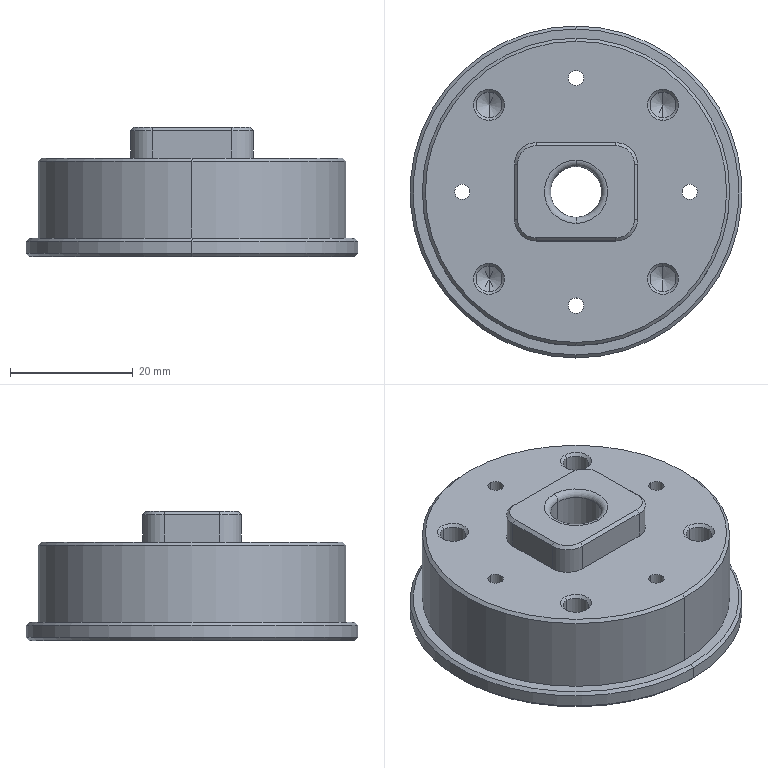NC program | NX | posted with a generic post | part box 54 x 54 x 21 mm
Lines 4215 to 5114 of 9691:
(ZLEVEL_PROFILE_1_COPY , TOOL : D4R0.5)
N8404 T17 M6
N8406 G54
N8408 G17 G0 G90 X-1.092 Y7.723 S9500 M3
N8410 G43 Z30. H17
N8412 Z-0.1
N8414 G94 G1 Z-1.6 F2500.
N8416 X-0.715 Y7.158
N8418 G3 X-0.356 Y6.981 R0.4
N8420 G1 X-0.055 Y7.
N8422 X0.105 Y6.999
N8424 X0.795 Y6.955
N8426 G2 X1.661 Y6.8 R15.853
N8428 G1 X1.824 Y6.758
N8430 X2.491 Y6.542
N8432 X2.656 Y6.477
N8434 X3.299 Y6.174
N8436 X3.391 Y6.123
N8438 X4.045 Y5.713
N8440 X4.129 Y5.652
N8442 X4.719 Y5.17
N8444 X4.804 Y5.091
N8446 X5.336 Y4.531
N8448 X5.445 Y4.399
N8450 X5.865 Y3.821
N8452 G2 X6.711 Y1.978 R7.418
N8454 X6.218 Y-3.201 R6.976
N8456 G1 X5.963 Y-3.665
N8458 G2 X5.445 Y-4.399 R14.342
N8460 G1 X5.37 Y-4.491
N8462 X4.862 Y-5.036
N8464 G2 X4.186 Y-5.611 R8.765
N8466 G1 X4.045 Y-5.713
N8468 X3.455 Y-6.088
N8470 X3.299 Y-6.174
N8472 X2.656 Y-6.477
N8474 X2.544 Y-6.521
N8476 X1.824 Y-6.758
N8478 X1.696 Y-6.791
N8480 X0.972 Y-6.932
N8482 X0.848 Y-6.948
N8484 X0.066 Y-7.
N8486 X-0.088 Y-6.998
N8488 X-0.795 Y-6.955
N8490 G2 X-1.787 Y-6.773 R15.853
N8492 G1 X-1.839 Y-6.752
N8494 X-2.491 Y-6.542
N8496 X-2.656 Y-6.477
N8498 X-3.299 Y-6.174
N8500 X-3.391 Y-6.123
N8502 X-4.045 Y-5.713
N8504 X-4.129 Y-5.652
N8506 X-4.719 Y-5.17
N8508 X-4.804 Y-5.091
N8510 X-5.336 Y-4.531
N8512 X-5.445 Y-4.399
N8514 X-5.855 Y-3.837
N8516 G2 X-6.71 Y-1.978 R7.402
N8518 X-6.218 Y3.202 R6.977
N8520 G1 X-5.963 Y3.665
N8522 G2 X-5.445 Y4.399 R13.396
N8524 G1 X-5.343 Y4.522
N8526 X-4.862 Y5.036
N8528 G2 X-4.186 Y5.611 R8.767
N8530 G1 X-4.045 Y5.713
N8532 X-3.455 Y6.088
N8534 X-3.299 Y6.174
N8536 X-2.656 Y6.477
N8538 X-2.544 Y6.521
N8540 X-1.824 Y6.758
N8542 X-1.696 Y6.791
N8544 X-0.972 Y6.932
N8546 X-0.848 Y6.948
N8548 X-0.356 Y6.981
N8550 X-0.22 Y6.991 Z-1.602
N8552 X-0.084 Y6.999 Z-1.605
N8554 X0.053 Z-1.607
N8556 X0.189 Y6.993 Z-1.61
N8558 X0.325 Y6.984 Z-1.612
N8560 X0.461 Y6.975 Z-1.614
N8562 X0.597 Y6.967 Z-1.617
N8564 X0.733 Y6.958 Z-1.619
N8566 X0.869 Y6.946 Z-1.621
N8568 X1.004 Y6.925 Z-1.624
N8570 X1.138 Y6.899 Z-1.626
N8572 X1.272 Y6.874 Z-1.629
N8574 X1.406 Y6.848 Z-1.631
N8576 X1.54 Y6.823 Z-1.633
N8578 X1.674 Y6.796 Z-1.636
N8580 X1.806 Y6.762 Z-1.638
N8582 X1.936 Y6.721 Z-1.64
N8584 X2.066 Y6.679 Z-1.643
N8586 X2.195 Y6.637 Z-1.645
N8588 X2.325 Y6.595 Z-1.648
N8590 X2.455 Y6.553 Z-1.65
N8592 X2.583 Y6.506 Z-1.652
N8594 X2.708 Y6.452 Z-1.655
N8596 X2.831 Y6.394 Z-1.657
N8598 X2.955 Y6.335 Z-1.66
N8600 X3.078 Y6.278 Z-1.662
N8602 X3.202 Y6.219 Z-1.664
N8604 X3.324 Y6.16 Z-1.667
N8606 X3.444 Y6.094 Z-1.669
N8608 X3.559 Y6.021 Z-1.671
N8610 X3.674 Y5.948 Z-1.674
N8612 X3.789 Y5.875 Z-1.676
N8614 X3.905 Y5.802 Z-1.679
N8616 X4.02 Y5.729 Z-1.681
N8618 X4.131 Y5.65 Z-1.683
N8620 X4.239 Y5.566 Z-1.686
N8622 X4.344 Y5.479 Z-1.688
N8624 X4.449 Y5.392 Z-1.69
N8626 X4.554 Y5.305 Z-1.693
N8628 X4.659 Y5.219 Z-1.695
N8630 X4.763 Y5.13 Z-1.698
N8632 X4.859 Y5.033 Z-1.7
N8634 X5.336 Y4.531
N8636 X5.445 Y4.399
N8638 X5.865 Y3.821
N8640 G2 X6.711 Y1.978 R7.414
N8642 X6.218 Y-3.202 R6.972
N8644 G1 X5.963 Y-3.665
N8646 G2 X5.445 Y-4.399 R14.292
N8648 G1 X5.37 Y-4.491
N8650 X4.862 Y-5.036
N8652 G2 X4.186 Y-5.611 R8.686
N8654 G1 X4.045 Y-5.713
N8656 X3.455 Y-6.088
N8658 X3.299 Y-6.174
N8660 X2.656 Y-6.477
N8662 X2.544 Y-6.521
N8664 X1.824 Y-6.758
N8666 X1.696 Y-6.791
N8668 X0.972 Y-6.932
N8670 X0.848 Y-6.948
N8672 X0.066 Y-7.
N8674 X-0.105 Y-6.999
N8676 X-0.795 Y-6.955
N8678 G2 X-1.786 Y-6.774 R15.853
N8680 G1 X-1.839 Y-6.752
N8682 X-2.491 Y-6.542
N8684 X-2.656 Y-6.477
N8686 X-3.299 Y-6.174
N8688 X-3.391 Y-6.123
N8690 X-4.045 Y-5.713
N8692 X-4.129 Y-5.652
N8694 X-4.719 Y-5.17
N8696 X-4.804 Y-5.091
N8698 X-5.336 Y-4.531
N8700 X-5.445 Y-4.399
N8702 X-5.855 Y-3.837
N8704 G2 X-6.71 Y-1.978 R7.4
N8706 X-6.218 Y3.202 R6.976
N8708 G1 X-5.963 Y3.665
N8710 G2 X-5.445 Y4.399 R13.397
N8712 G1 X-5.37 Y4.491
N8714 X-4.862 Y5.036
N8716 G2 X-4.186 Y5.611 R8.688
N8718 G1 X-4.045 Y5.713
N8720 X-3.455 Y6.088
N8722 X-3.299 Y6.174
N8724 X-2.656 Y6.477
N8726 X-2.544 Y6.521
N8728 X-1.824 Y6.758
N8730 X-1.696 Y6.791
N8732 X-0.972 Y6.932
N8734 X-0.848 Y6.948
N8736 X-0.356 Y6.981
N8738 X-0.22 Y6.991 Z-1.702
N8740 X-0.084 Y6.999 Z-1.705
N8742 X0.053 Z-1.707
N8744 X0.189 Y6.993 Z-1.71
N8746 X0.325 Y6.984 Z-1.712
N8748 X0.461 Y6.975 Z-1.714
N8750 X0.597 Y6.967 Z-1.717
N8752 X0.733 Y6.959 Z-1.719
N8754 X0.869 Y6.945 Z-1.721
N8756 X1.004 Y6.925 Z-1.724
N8758 X1.138 Y6.9 Z-1.726
N8760 X1.272 Y6.874 Z-1.729
N8762 X1.406 Y6.848 Z-1.731
N8764 X1.54 Y6.823 Z-1.733
N8766 X1.674 Y6.796 Z-1.736
N8768 X1.806 Y6.762 Z-1.738
N8770 X1.936 Y6.721 Z-1.74
N8772 X2.066 Y6.68 Z-1.743
N8774 X2.195 Y6.637 Z-1.745
N8776 X2.325 Y6.595 Z-1.748
N8778 X2.455 Y6.553 Z-1.75
N8780 X2.583 Y6.506 Z-1.752
N8782 X2.708 Y6.452 Z-1.755
N8784 X2.831 Y6.394 Z-1.757
N8786 X2.955 Y6.335 Z-1.76
N8788 X3.078 Y6.278 Z-1.762
N8790 X3.202 Y6.22 Z-1.764
N8792 X3.324 Y6.16 Z-1.767
N8794 X3.444 Y6.094 Z-1.769
N8796 X3.559 Y6.021 Z-1.771
N8798 X3.674 Y5.948 Z-1.774
N8800 X3.789 Y5.875 Z-1.776
N8802 X3.905 Y5.802 Z-1.779
N8804 X4.02 Y5.729 Z-1.781
N8806 X4.131 Y5.65 Z-1.783
N8808 X4.239 Y5.566 Z-1.786
N8810 X4.344 Y5.479 Z-1.788
N8812 X4.449 Y5.392 Z-1.79
N8814 X4.554 Y5.305 Z-1.793
N8816 X4.659 Y5.219 Z-1.795
N8818 X4.763 Y5.13 Z-1.798
N8820 X4.859 Y5.033 Z-1.8
N8822 X5.336 Y4.531
N8824 X5.445 Y4.399
N8826 X5.865 Y3.821
N8828 G2 X6.711 Y1.978 R7.408
N8830 X6.218 Y-3.202 R6.972
N8832 G1 X5.963 Y-3.665
N8834 G2 X5.445 Y-4.399 R14.155
N8836 G1 X5.37 Y-4.491
N8838 X4.862 Y-5.036
N8840 G2 X4.186 Y-5.611 R8.61
N8842 G1 X4.045 Y-5.713
N8844 X3.455 Y-6.088
N8846 X3.299 Y-6.174
N8848 X2.656 Y-6.477
N8850 X2.544 Y-6.521
N8852 X1.824 Y-6.758
N8854 X1.696 Y-6.791
N8856 X0.972 Y-6.932
N8858 X0.848 Y-6.948
N8860 X0.066 Y-7.
N8862 X-0.105 Y-6.999
N8864 X-0.795 Y-6.955
N8866 G2 X-1.785 Y-6.774 R15.853
N8868 G1 X-1.839 Y-6.752
N8870 X-2.491 Y-6.542
N8872 X-2.656 Y-6.477
N8874 X-3.299 Y-6.174
N8876 X-3.391 Y-6.123
N8878 X-4.045 Y-5.713
N8880 X-4.129 Y-5.652
N8882 X-4.719 Y-5.17
N8884 X-4.804 Y-5.091
N8886 X-5.336 Y-4.531
N8888 X-5.445 Y-4.399
N8890 X-5.855 Y-3.837
N8892 G2 X-6.711 Y-1.978 R7.395
N8894 X-6.218 Y3.202 R6.969
N8896 G1 X-5.963 Y3.665
N8898 G2 X-5.445 Y4.399 R13.399
N8900 G1 X-5.37 Y4.491
N8902 X-4.862 Y5.036
N8904 G2 X-4.186 Y5.611 R8.612
N8906 G1 X-4.045 Y5.713
N8908 X-3.455 Y6.088
N8910 X-3.299 Y6.174
N8912 X-2.656 Y6.477
N8914 X-2.544 Y6.521
N8916 X-1.824 Y6.758
N8918 X-1.696 Y6.791
N8920 X-0.972 Y6.932
N8922 X-0.848 Y6.948
N8924 X-0.356 Y6.981
N8926 X-0.22 Y6.991 Z-1.802
N8928 X-0.084 Y6.999 Z-1.805
N8930 X0.053 Y7. Z-1.807
N8932 X0.189 Y6.993 Z-1.81
N8934 X0.325 Y6.984 Z-1.812
N8936 X0.461 Y6.975 Z-1.814
N8938 X0.597 Y6.967 Z-1.817
N8940 X0.733 Y6.958 Z-1.819
N8942 X0.869 Y6.945 Z-1.821
N8944 X1.004 Y6.925 Z-1.824
N8946 X1.138 Y6.9 Z-1.826
N8948 X1.272 Y6.874 Z-1.829
N8950 X1.406 Y6.848 Z-1.831
N8952 X1.54 Y6.823 Z-1.833
N8954 X1.674 Y6.796 Z-1.836
N8956 X1.806 Y6.762 Z-1.838
N8958 X1.936 Y6.721 Z-1.84
N8960 X2.066 Y6.68 Z-1.843
N8962 X2.195 Y6.637 Z-1.845
N8964 X2.325 Y6.595 Z-1.848
N8966 X2.455 Y6.553 Z-1.85
N8968 X2.583 Y6.506 Z-1.852
N8970 X2.708 Y6.452 Z-1.855
N8972 X2.831 Y6.394 Z-1.857
N8974 X2.955 Y6.336 Z-1.86
N8976 X3.078 Y6.278 Z-1.862
N8978 X3.202 Y6.22 Z-1.864
N8980 X3.324 Y6.16 Z-1.867
N8982 X3.444 Y6.094 Z-1.869
N8984 X3.559 Y6.021 Z-1.871
N8986 X3.674 Y5.948 Z-1.874
N8988 X3.789 Y5.875 Z-1.876
N8990 X3.905 Y5.802 Z-1.879
N8992 X4.02 Y5.729 Z-1.881
N8994 X4.131 Y5.65 Z-1.883
N8996 X4.239 Y5.566 Z-1.886
N8998 X4.344 Y5.48 Z-1.888
N9000 X4.449 Y5.392 Z-1.89
N9002 X4.554 Y5.305 Z-1.893
N9004 X4.659 Y5.219 Z-1.895
N9006 X4.763 Y5.13 Z-1.898
N9008 X4.859 Y5.033 Z-1.9
N9010 X5.336 Y4.531
N9012 X5.445 Y4.399
N9014 X5.865 Y3.821
N9016 G2 X6.711 Y1.978 R7.402
N9018 X6.218 Y-3.202 R6.972
N9020 G1 X5.963 Y-3.665
N9022 G2 X5.445 Y-4.399 R14.021
N9024 G1 X5.37 Y-4.491
N9026 X4.862 Y-5.036
N9028 G2 X3.755 Y-5.919 R8.534
N9030 X2.656 Y-6.477 R10.668
N9032 G1 X2.544 Y-6.521
N9034 X1.824 Y-6.758
N9036 X1.696 Y-6.791
N9038 X0.972 Y-6.932
N9040 X0.848 Y-6.948
N9042 X0.066 Y-7.
N9044 X-0.105 Y-6.999
N9046 X-0.795 Y-6.955
N9048 G2 X-1.783 Y-6.774 R15.853
N9050 G1 X-1.839 Y-6.752
N9052 X-2.491 Y-6.542
N9054 X-2.656 Y-6.477
N9056 X-3.299 Y-6.174
N9058 X-3.391 Y-6.123
N9060 X-4.045 Y-5.713
N9062 X-4.129 Y-5.652
N9064 X-4.719 Y-5.17
N9066 X-4.804 Y-5.091
N9068 X-5.336 Y-4.531
N9070 X-5.445 Y-4.399
N9072 X-5.855 Y-3.837
N9074 G2 X-6.711 Y-1.978 R7.398
N9076 X-6.218 Y3.202 R6.971
N9078 G1 X-5.963 Y3.665
N9080 G2 X-5.445 Y4.399 R13.4
N9082 G1 X-5.37 Y4.491
N9084 X-4.862 Y5.036
N9086 G2 X-3.755 Y5.919 R8.536
N9088 X-2.656 Y6.477 R10.667
N9090 G1 X-2.544 Y6.521
N9092 X-1.824 Y6.758
N9094 X-1.696 Y6.791
N9096 X-0.972 Y6.932
N9098 X-0.848 Y6.948
N9100 X-0.356 Y6.981
N9102 X-0.22 Y6.991 Z-1.902
N9104 X-0.084 Y6.999 Z-1.905
N9106 X0.052 Z-1.907
N9108 X0.189 Y6.993 Z-1.91
N9110 X0.325 Y6.985 Z-1.912
N9112 X0.461 Y6.977 Z-1.914
N9114 X0.597 Y6.967 Z-1.917
N9116 X0.733 Y6.958 Z-1.919
N9118 X0.869 Y6.945 Z-1.921
N9120 X1.004 Y6.925 Z-1.924
N9122 X1.138 Y6.901 Z-1.926
N9124 X1.273 Y6.878 Z-1.929
N9126 X1.407 Y6.852 Z-1.931
N9128 X1.54 Y6.824 Z-1.933
N9130 X1.674 Y6.797 Z-1.936
N9132 X1.806 Y6.763 Z-1.938
N9134 X1.936 Y6.723 Z-1.94
N9136 X2.067 Y6.684 Z-1.943
N9138 X2.197 Y6.643 Z-1.945
N9140 X2.326 Y6.599 Z-1.948
N9142 X2.455 Y6.553 Z-1.95
N9144 X2.583 Y6.506 Z-1.952
N9146 X2.708 Y6.453 Z-1.955
N9148 X2.834 Y6.399 Z-1.957
N9150 X2.958 Y6.343 Z-1.96
N9152 X3.081 Y6.284 Z-1.962
N9154 X3.203 Y6.223 Z-1.964
N9156 X3.324 Y6.16 Z-1.967
N9158 X3.444 Y6.094 Z-1.969
N9160 X3.562 Y6.025 Z-1.971
N9162 X3.678 Y5.955 Z-1.974
N9164 X3.794 Y5.882 Z-1.976
N9166 X3.908 Y5.807 Z-1.979
N9168 X4.02 Y5.73 Z-1.981
N9170 X4.131 Y5.65 Z-1.983
N9172 X4.241 Y5.569 Z-1.986
N9174 X4.348 Y5.485 Z-1.988
N9176 X4.455 Y5.399 Z-1.99
N9178 X4.559 Y5.312 Z-1.993
N9180 X4.662 Y5.221 Z-1.995
N9182 X4.762 Y5.129 Z-1.998
N9184 X4.862 Y5.036 Z-2.
N9186 G2 X-0.357 Y6.991 R-7.
N9188 G1 X-0.22 Y6.997 Z-2.002
N9190 X-0.084 Y6.999 Z-2.005
N9192 X0.053 Y7. Z-2.007
N9194 X0.189 Y6.997 Z-2.01
N9196 X0.325 Y6.992 Z-2.012
N9198 X0.461 Y6.985 Z-2.014
N9200 X0.597 Y6.974 Z-2.017
N9202 X0.733 Y6.961 Z-2.019
N9204 X0.869 Y6.946 Z-2.021
N9206 X1.004 Y6.928 Z-2.024
N9208 X1.139 Y6.907 Z-2.026
N9210 X1.273 Y6.883 Z-2.029
N9212 X1.407 Y6.857 Z-2.031
N9214 X1.54 Y6.828 Z-2.033
N9216 X1.673 Y6.797 Z-2.036
N9218 X1.805 Y6.763 Z-2.038
N9220 X1.937 Y6.727 Z-2.04
N9222 X2.067 Y6.688 Z-2.043
N9224 X2.197 Y6.646 Z-2.045
N9226 X2.326 Y6.602 Z-2.048
N9228 X2.455 Y6.556 Z-2.05
N9230 X2.582 Y6.506 Z-2.052
N9232 X2.708 Y6.455 Z-2.055
N9234 X2.833 Y6.401 Z-2.057
N9236 X2.958 Y6.345 Z-2.06
N9238 X3.081 Y6.286 Z-2.062
N9240 X3.202 Y6.224 Z-2.064
N9242 X3.323 Y6.161 Z-2.067
N9244 X3.443 Y6.095 Z-2.069
N9246 X3.561 Y6.027 Z-2.071
N9248 X3.677 Y5.956 Z-2.074
N9250 X3.793 Y5.883 Z-2.076
N9252 X3.907 Y5.808 Z-2.079
N9254 X4.019 Y5.731 Z-2.081
N9256 X4.13 Y5.652 Z-2.083
N9258 X4.239 Y5.57 Z-2.086
N9260 X4.347 Y5.487 Z-2.088
N9262 X4.453 Y5.401 Z-2.09
N9264 X4.558 Y5.313 Z-2.093
N9266 X4.66 Y5.223 Z-2.095
N9268 X4.761 Y5.131 Z-2.098
N9270 X4.86 Y5.038 Z-2.1
N9272 G2 X-0.357 Y6.991 R-7.
N9274 G1 X-0.22 Y6.997 Z-2.102
N9276 X-0.084 Y6.999 Z-2.105
N9278 X0.053 Y7. Z-2.107
N9280 X0.189 Y6.997 Z-2.11
N9282 X0.325 Y6.992 Z-2.112
N9284 X0.461 Y6.985 Z-2.114
N9286 X0.597 Y6.974 Z-2.117
N9288 X0.733 Y6.961 Z-2.119
N9290 X0.869 Y6.946 Z-2.121
N9292 X1.004 Y6.928 Z-2.124
N9294 X1.139 Y6.907 Z-2.126
N9296 X1.273 Y6.883 Z-2.129
N9298 X1.407 Y6.857 Z-2.131
N9300 X1.54 Y6.828 Z-2.133
N9302 X1.673 Y6.797 Z-2.136
N9304 X1.805 Y6.763 Z-2.138
N9306 X1.937 Y6.727 Z-2.14
N9308 X2.067 Y6.688 Z-2.143
N9310 X2.197 Y6.646 Z-2.145
N9312 X2.326 Y6.602 Z-2.148
N9314 X2.455 Y6.556 Z-2.15
N9316 X2.582 Y6.506 Z-2.152
N9318 X2.708 Y6.455 Z-2.155
N9320 X2.833 Y6.401 Z-2.157
N9322 X2.958 Y6.345 Z-2.16
N9324 X3.081 Y6.286 Z-2.162
N9326 X3.202 Y6.224 Z-2.164
N9328 X3.323 Y6.161 Z-2.167
N9330 X3.443 Y6.095 Z-2.169
N9332 X3.561 Y6.027 Z-2.171
N9334 X3.677 Y5.956 Z-2.174
N9336 X3.793 Y5.883 Z-2.176
N9338 X3.907 Y5.808 Z-2.179
N9340 X4.019 Y5.731 Z-2.181
N9342 X4.13 Y5.652 Z-2.183
N9344 X4.239 Y5.57 Z-2.186
N9346 X4.347 Y5.487 Z-2.188
N9348 X4.453 Y5.401 Z-2.19
N9350 X4.558 Y5.313 Z-2.193
N9352 X4.66 Y5.223 Z-2.195
N9354 X4.761 Y5.131 Z-2.198
N9356 X4.86 Y5.038 Z-2.2
N9358 G2 X-0.357 Y6.991 R-7.
N9360 G1 X-0.22 Y6.997 Z-2.202
N9362 X-0.084 Y6.999 Z-2.205
N9364 X0.053 Y7. Z-2.207
N9366 X0.189 Y6.997 Z-2.21
N9368 X0.325 Y6.992 Z-2.212
N9370 X0.461 Y6.985 Z-2.214
N9372 X0.597 Y6.974 Z-2.217
N9374 X0.733 Y6.961 Z-2.219
N9376 X0.869 Y6.946 Z-2.221
N9378 X1.004 Y6.928 Z-2.224
N9380 X1.139 Y6.907 Z-2.226
N9382 X1.273 Y6.883 Z-2.229
N9384 X1.407 Y6.857 Z-2.231
N9386 X1.54 Y6.828 Z-2.233
N9388 X1.673 Y6.797 Z-2.236
N9390 X1.805 Y6.763 Z-2.238
N9392 X1.937 Y6.727 Z-2.24
N9394 X2.067 Y6.688 Z-2.243
N9396 X2.197 Y6.646 Z-2.245
N9398 X2.326 Y6.602 Z-2.248
N9400 X2.455 Y6.556 Z-2.25
N9402 X2.582 Y6.506 Z-2.252
N9404 X2.708 Y6.455 Z-2.255
N9406 X2.833 Y6.401 Z-2.257
N9408 X2.958 Y6.345 Z-2.26
N9410 X3.081 Y6.286 Z-2.262
N9412 X3.202 Y6.224 Z-2.264
N9414 X3.323 Y6.161 Z-2.267
N9416 X3.443 Y6.095 Z-2.269
N9418 X3.561 Y6.027 Z-2.271
N9420 X3.677 Y5.956 Z-2.274
N9422 X3.793 Y5.883 Z-2.276
N9424 X3.907 Y5.808 Z-2.279
N9426 X4.019 Y5.731 Z-2.281
N9428 X4.13 Y5.652 Z-2.283
N9430 X4.239 Y5.57 Z-2.286
N9432 X4.347 Y5.487 Z-2.288
N9434 X4.453 Y5.401 Z-2.29
N9436 X4.558 Y5.313 Z-2.293
N9438 X4.66 Y5.223 Z-2.295
N9440 X4.761 Y5.131 Z-2.298
N9442 X4.86 Y5.038 Z-2.3
N9444 G2 X-0.357 Y6.991 R-7.
N9446 G1 X-0.22 Y6.997 Z-2.302
N9448 X-0.084 Y6.999 Z-2.305
N9450 X0.053 Y7. Z-2.307
N9452 X0.189 Y6.997 Z-2.31
N9454 X0.325 Y6.992 Z-2.312
N9456 X0.461 Y6.985 Z-2.314
N9458 X0.597 Y6.974 Z-2.317
N9460 X0.733 Y6.961 Z-2.319
N9462 X0.869 Y6.946 Z-2.321
N9464 X1.004 Y6.928 Z-2.324
N9466 X1.139 Y6.907 Z-2.326
N9468 X1.273 Y6.883 Z-2.329
N9470 X1.407 Y6.857 Z-2.331
N9472 X1.54 Y6.828 Z-2.333
N9474 X1.673 Y6.797 Z-2.336
N9476 X1.805 Y6.763 Z-2.338
N9478 X1.937 Y6.727 Z-2.34
N9480 X2.067 Y6.688 Z-2.343
N9482 X2.197 Y6.646 Z-2.345
N9484 X2.326 Y6.602 Z-2.348
N9486 X2.455 Y6.556 Z-2.35
N9488 X2.582 Y6.506 Z-2.352
N9490 X2.708 Y6.455 Z-2.355
N9492 X2.833 Y6.401 Z-2.357
N9494 X2.958 Y6.345 Z-2.36
N9496 X3.081 Y6.286 Z-2.362
N9498 X3.202 Y6.224 Z-2.364
N9500 X3.323 Y6.161 Z-2.367
N9502 X3.443 Y6.095 Z-2.369
N9504 X3.561 Y6.027 Z-2.371
N9506 X3.677 Y5.956 Z-2.374
N9508 X3.793 Y5.883 Z-2.376
N9510 X3.907 Y5.808 Z-2.379
N9512 X4.019 Y5.731 Z-2.381
N9514 X4.13 Y5.652 Z-2.383
N9516 X4.239 Y5.57 Z-2.386
N9518 X4.347 Y5.487 Z-2.388
N9520 X4.453 Y5.401 Z-2.39
N9522 X4.558 Y5.313 Z-2.393
N9524 X4.66 Y5.223 Z-2.395
N9526 X4.761 Y5.131 Z-2.398
N9528 X4.86 Y5.038 Z-2.4
N9530 G2 X-0.357 Y6.991 R-7.
N9532 G1 X-0.22 Y6.997 Z-2.402
N9534 X-0.084 Y6.999 Z-2.405
N9536 X0.053 Y7. Z-2.407
N9538 X0.189 Y6.997 Z-2.41
N9540 X0.325 Y6.992 Z-2.412
N9542 X0.461 Y6.985 Z-2.414
N9544 X0.597 Y6.974 Z-2.417
N9546 X0.733 Y6.961 Z-2.419
N9548 X0.869 Y6.946 Z-2.421
N9550 X1.004 Y6.928 Z-2.424
N9552 X1.139 Y6.907 Z-2.426
N9554 X1.273 Y6.883 Z-2.429
N9556 X1.407 Y6.857 Z-2.431
N9558 X1.54 Y6.828 Z-2.433
N9560 X1.673 Y6.797 Z-2.436
N9562 X1.805 Y6.763 Z-2.438
N9564 X1.937 Y6.727 Z-2.44
N9566 X2.067 Y6.688 Z-2.443
N9568 X2.197 Y6.646 Z-2.445
N9570 X2.326 Y6.602 Z-2.448
N9572 X2.455 Y6.556 Z-2.45
N9574 X2.582 Y6.506 Z-2.452
N9576 X2.708 Y6.455 Z-2.455
N9578 X2.833 Y6.401 Z-2.457
N9580 X2.958 Y6.345 Z-2.46
N9582 X3.081 Y6.286 Z-2.462
N9584 X3.202 Y6.224 Z-2.464
N9586 X3.323 Y6.161 Z-2.467
N9588 X3.443 Y6.095 Z-2.469
N9590 X3.561 Y6.027 Z-2.471
N9592 X3.677 Y5.956 Z-2.474
N9594 X3.793 Y5.883 Z-2.476
N9596 X3.907 Y5.808 Z-2.479
N9598 X4.019 Y5.731 Z-2.481
N9600 X4.13 Y5.652 Z-2.483
N9602 X4.239 Y5.57 Z-2.486
N9604 X4.347 Y5.487 Z-2.488
N9606 X4.453 Y5.401 Z-2.49
N9608 X4.558 Y5.313 Z-2.493
N9610 X4.66 Y5.223 Z-2.495
N9612 X4.761 Y5.131 Z-2.498
N9614 X4.86 Y5.038 Z-2.5
N9616 G2 X-0.357 Y6.991 R-7.
N9618 G1 X-0.22 Y6.997 Z-2.502
N9620 X-0.084 Y6.999 Z-2.505
N9622 X0.053 Y7. Z-2.507
N9624 X0.189 Y6.997 Z-2.51
N9626 X0.325 Y6.992 Z-2.512
N9628 X0.461 Y6.985 Z-2.514
N9630 X0.597 Y6.974 Z-2.517
N9632 X0.733 Y6.961 Z-2.519
N9634 X0.869 Y6.946 Z-2.521
N9636 X1.004 Y6.928 Z-2.524
N9638 X1.139 Y6.907 Z-2.526
N9640 X1.273 Y6.883 Z-2.529
N9642 X1.407 Y6.857 Z-2.531
N9644 X1.54 Y6.828 Z-2.533
N9646 X1.673 Y6.797 Z-2.536
N9648 X1.805 Y6.763 Z-2.538
N9650 X1.937 Y6.727 Z-2.54
N9652 X2.067 Y6.688 Z-2.543
N9654 X2.197 Y6.646 Z-2.545
N9656 X2.326 Y6.602 Z-2.548
N9658 X2.455 Y6.556 Z-2.55
N9660 X2.582 Y6.506 Z-2.552
N9662 X2.708 Y6.455 Z-2.555
N9664 X2.833 Y6.401 Z-2.557
N9666 X2.958 Y6.345 Z-2.56
N9668 X3.081 Y6.286 Z-2.562
N9670 X3.202 Y6.224 Z-2.564
N9672 X3.323 Y6.161 Z-2.567
N9674 X3.443 Y6.095 Z-2.569
N9676 X3.561 Y6.027 Z-2.571
N9678 X3.677 Y5.956 Z-2.574
N9680 X3.793 Y5.883 Z-2.576
N9682 X3.907 Y5.808 Z-2.579
N9684 X4.019 Y5.731 Z-2.581
N9686 X4.13 Y5.652 Z-2.583
N9688 X4.239 Y5.57 Z-2.586
N9690 X4.347 Y5.487 Z-2.588
N9692 X4.453 Y5.401 Z-2.59
N9694 X4.558 Y5.313 Z-2.593
N9696 X4.66 Y5.223 Z-2.595
N9698 X4.761 Y5.131 Z-2.598
N9700 X4.86 Y5.038 Z-2.6
N9702 G2 X-0.357 Y6.991 R-7.
N9704 G1 X-0.22 Y6.997 Z-2.602
N9706 X-0.084 Y6.999 Z-2.605
N9708 X0.053 Y7. Z-2.607
N9710 X0.189 Y6.997 Z-2.61
N9712 X0.325 Y6.992 Z-2.612
N9714 X0.461 Y6.985 Z-2.614
N9716 X0.597 Y6.974 Z-2.617
N9718 X0.733 Y6.961 Z-2.619
N9720 X0.869 Y6.946 Z-2.621
N9722 X1.004 Y6.928 Z-2.624
N9724 X1.139 Y6.907 Z-2.626
N9726 X1.273 Y6.883 Z-2.629
N9728 X1.407 Y6.857 Z-2.631
N9730 X1.54 Y6.828 Z-2.633
N9732 X1.673 Y6.797 Z-2.636
N9734 X1.805 Y6.763 Z-2.638
N9736 X1.937 Y6.727 Z-2.64
N9738 X2.067 Y6.688 Z-2.643
N9740 X2.197 Y6.646 Z-2.645
N9742 X2.326 Y6.602 Z-2.648
N9744 X2.455 Y6.556 Z-2.65
N9746 X2.582 Y6.506 Z-2.652
N9748 X2.708 Y6.455 Z-2.655
N9750 X2.833 Y6.401 Z-2.657
N9752 X2.958 Y6.345 Z-2.66
N9754 X3.081 Y6.286 Z-2.662
N9756 X3.202 Y6.224 Z-2.664
N9758 X3.323 Y6.161 Z-2.667
N9760 X3.443 Y6.095 Z-2.669
N9762 X3.561 Y6.027 Z-2.671
N9764 X3.677 Y5.956 Z-2.674
N9766 X3.793 Y5.883 Z-2.676
N9768 X3.907 Y5.808 Z-2.679
N9770 X4.019 Y5.731 Z-2.681
N9772 X4.13 Y5.652 Z-2.683
N9774 X4.239 Y5.57 Z-2.686
N9776 X4.347 Y5.487 Z-2.688
N9778 X4.453 Y5.401 Z-2.69
N9780 X4.558 Y5.313 Z-2.693
N9782 X4.66 Y5.223 Z-2.695
N9784 X4.761 Y5.131 Z-2.698
N9786 X4.86 Y5.038 Z-2.7
N9788 G2 X-0.357 Y6.991 R-7.
N9790 G1 X-0.22 Y6.997 Z-2.702
N9792 X-0.084 Y6.999 Z-2.705
N9794 X0.053 Y7. Z-2.707
N9796 X0.189 Y6.997 Z-2.71
N9798 X0.325 Y6.992 Z-2.712
N9800 X0.461 Y6.985 Z-2.714
N9802 X0.597 Y6.974 Z-2.717
N9804 X0.733 Y6.961 Z-2.719
N9806 X0.869 Y6.946 Z-2.721
N9808 X1.004 Y6.928 Z-2.724
N9810 X1.139 Y6.907 Z-2.726
N9812 X1.273 Y6.883 Z-2.729
N9814 X1.407 Y6.857 Z-2.731
N9816 X1.54 Y6.828 Z-2.733
N9818 X1.673 Y6.797 Z-2.736
N9820 X1.805 Y6.763 Z-2.738
N9822 X1.937 Y6.727 Z-2.74
N9824 X2.067 Y6.688 Z-2.743
N9826 X2.197 Y6.646 Z-2.745
N9828 X2.326 Y6.602 Z-2.748
N9830 X2.455 Y6.556 Z-2.75
N9832 X2.582 Y6.506 Z-2.752
N9834 X2.708 Y6.455 Z-2.755
N9836 X2.833 Y6.401 Z-2.757
N9838 X2.958 Y6.345 Z-2.76
N9840 X3.081 Y6.286 Z-2.762
N9842 X3.202 Y6.224 Z-2.764
N9844 X3.323 Y6.161 Z-2.767
N9846 X3.443 Y6.095 Z-2.769
N9848 X3.561 Y6.027 Z-2.771
N9850 X3.677 Y5.956 Z-2.774
N9852 X3.793 Y5.883 Z-2.776
N9854 X3.907 Y5.808 Z-2.779
N9856 X4.019 Y5.731 Z-2.781
N9858 X4.13 Y5.652 Z-2.783
N9860 X4.239 Y5.57 Z-2.786
N9862 X4.347 Y5.487 Z-2.788
N9864 X4.453 Y5.401 Z-2.79
N9866 X4.558 Y5.313 Z-2.793
N9868 X4.66 Y5.223 Z-2.795
N9870 X4.761 Y5.131 Z-2.798
N9872 X4.86 Y5.038 Z-2.8
N9874 G2 X-0.357 Y6.991 R-7.
N9876 G1 X-0.22 Y6.997 Z-2.802
N9878 X-0.084 Y6.999 Z-2.805
N9880 X0.053 Y7. Z-2.807
N9882 X0.189 Y6.997 Z-2.81
N9884 X0.325 Y6.992 Z-2.812
N9886 X0.461 Y6.985 Z-2.814
N9888 X0.597 Y6.974 Z-2.817
N9890 X0.733 Y6.961 Z-2.819
N9892 X0.869 Y6.946 Z-2.821
N9894 X1.004 Y6.928 Z-2.824
N9896 X1.139 Y6.907 Z-2.826
N9898 X1.273 Y6.883 Z-2.829
N9900 X1.407 Y6.857 Z-2.831
N9902 X1.54 Y6.828 Z-2.833
N9904 X1.673 Y6.797 Z-2.836
N9906 X1.805 Y6.763 Z-2.838
N9908 X1.937 Y6.727 Z-2.84
N9910 X2.067 Y6.688 Z-2.843
N9912 X2.197 Y6.646 Z-2.845
N9914 X2.326 Y6.602 Z-2.848
N9916 X2.455 Y6.556 Z-2.85
N9918 X2.582 Y6.506 Z-2.852
N9920 X2.708 Y6.455 Z-2.855
N9922 X2.833 Y6.401 Z-2.857
N9924 X2.958 Y6.345 Z-2.86
N9926 X3.081 Y6.286 Z-2.862
N9928 X3.202 Y6.224 Z-2.864
N9930 X3.323 Y6.161 Z-2.867
N9932 X3.443 Y6.095 Z-2.869
N9934 X3.561 Y6.027 Z-2.871
N9936 X3.677 Y5.956 Z-2.874
N9938 X3.793 Y5.883 Z-2.876
N9940 X3.907 Y5.808 Z-2.879
N9942 X4.019 Y5.731 Z-2.881
N9944 X4.13 Y5.652 Z-2.883
N9946 X4.239 Y5.57 Z-2.886
N9948 X4.347 Y5.487 Z-2.888
N9950 X4.453 Y5.401 Z-2.89
N9952 X4.558 Y5.313 Z-2.893
N9954 X4.66 Y5.223 Z-2.895
N9956 X4.761 Y5.131 Z-2.898
N9958 X4.86 Y5.038 Z-2.9
N9960 G2 X-0.357 Y6.991 R-7.
N9962 G1 X-0.22 Y6.997 Z-2.902
N9964 X-0.084 Y6.999 Z-2.905
N9966 X0.053 Y7. Z-2.907
N9968 X0.189 Y6.997 Z-2.91
N9970 X0.325 Y6.992 Z-2.912
N9972 X0.461 Y6.985 Z-2.914
N9974 X0.597 Y6.974 Z-2.917
N9976 X0.733 Y6.961 Z-2.919
N9978 X0.869 Y6.946 Z-2.921
N9980 X1.004 Y6.928 Z-2.924
N9982 X1.139 Y6.907 Z-2.926
N9984 X1.273 Y6.883 Z-2.929
N9986 X1.407 Y6.857 Z-2.931
N9988 X1.54 Y6.828 Z-2.933
N9990 X1.673 Y6.797 Z-2.936
N9992 X1.805 Y6.763 Z-2.938
N9994 X1.937 Y6.727 Z-2.94
N9996 X2.067 Y6.688 Z-2.943
N9998 X2.197 Y6.646 Z-2.945
N10000 X2.326 Y6.602 Z-2.948
N10002 X2.455 Y6.556 Z-2.95
N10004 X2.582 Y6.506 Z-2.952
N10006 X2.708 Y6.455 Z-2.955
N10008 X2.833 Y6.401 Z-2.957
N10010 X2.958 Y6.345 Z-2.96
N10012 X3.081 Y6.286 Z-2.962
N10014 X3.202 Y6.224 Z-2.964
N10016 X3.323 Y6.161 Z-2.967
N10018 X3.443 Y6.095 Z-2.969
N10020 X3.561 Y6.027 Z-2.971
N10022 X3.677 Y5.956 Z-2.974
N10024 X3.793 Y5.883 Z-2.976
N10026 X3.907 Y5.808 Z-2.979
N10028 X4.019 Y5.731 Z-2.981
N10030 X4.13 Y5.652 Z-2.983
N10032 X4.239 Y5.57 Z-2.986
N10034 X4.347 Y5.487 Z-2.988
N10036 X4.453 Y5.401 Z-2.99
N10038 X4.558 Y5.313 Z-2.993
N10040 X4.66 Y5.223 Z-2.995
N10042 X4.761 Y5.131 Z-2.998
N10044 X4.86 Y5.038 Z-3.
N10046 G2 X-0.357 Y6.991 R-7.
N10048 G1 X-0.22 Y6.997 Z-3.002
N10050 X-0.084 Y6.999 Z-3.005
N10052 X0.053 Y7. Z-3.007
N10054 X0.189 Y6.997 Z-3.01
N10056 X0.325 Y6.992 Z-3.012
N10058 X0.461 Y6.985 Z-3.014
N10060 X0.597 Y6.974 Z-3.017
N10062 X0.733 Y6.961 Z-3.019
N10064 X0.869 Y6.946 Z-3.021
N10066 X1.004 Y6.928 Z-3.024
N10068 X1.139 Y6.907 Z-3.026
N10070 X1.273 Y6.883 Z-3.029
N10072 X1.407 Y6.857 Z-3.031
N10074 X1.54 Y6.828 Z-3.033
N10076 X1.673 Y6.797 Z-3.036
N10078 X1.805 Y6.763 Z-3.038
N10080 X1.937 Y6.727 Z-3.04
N10082 X2.067 Y6.688 Z-3.043
N10084 X2.197 Y6.646 Z-3.045
N10086 X2.326 Y6.602 Z-3.048
N10088 X2.455 Y6.556 Z-3.05
N10090 X2.582 Y6.506 Z-3.052
N10092 X2.708 Y6.455 Z-3.055
N10094 X2.833 Y6.401 Z-3.057
N10096 X2.958 Y6.345 Z-3.06
N10098 X3.081 Y6.286 Z-3.062
N10100 X3.202 Y6.224 Z-3.064
N10102 X3.323 Y6.161 Z-3.067
N10104 X3.443 Y6.095 Z-3.069
N10106 X3.561 Y6.027 Z-3.071
N10108 X3.677 Y5.956 Z-3.074
N10110 X3.793 Y5.883 Z-3.076
N10112 X3.907 Y5.808 Z-3.079
N10114 X4.019 Y5.731 Z-3.081
N10116 X4.13 Y5.652 Z-3.083
N10118 X4.239 Y5.57 Z-3.086
N10120 X4.347 Y5.487 Z-3.088
N10122 X4.453 Y5.401 Z-3.09
N10124 X4.558 Y5.313 Z-3.093
N10126 X4.66 Y5.223 Z-3.095
N10128 X4.761 Y5.131 Z-3.098
N10130 X4.86 Y5.038 Z-3.1
N10132 G2 X-0.357 Y6.991 R-7.
N10134 G1 X-0.22 Y6.997 Z-3.102
N10136 X-0.084 Y6.999 Z-3.105
N10138 X0.053 Y7. Z-3.107
N10140 X0.189 Y6.997 Z-3.11
N10142 X0.325 Y6.992 Z-3.112
N10144 X0.461 Y6.985 Z-3.114
N10146 X0.597 Y6.974 Z-3.117
N10148 X0.733 Y6.961 Z-3.119
N10150 X0.869 Y6.946 Z-3.121
N10152 X1.004 Y6.928 Z-3.124
N10154 X1.139 Y6.907 Z-3.126
N10156 X1.273 Y6.883 Z-3.129
N10158 X1.407 Y6.857 Z-3.131
N10160 X1.54 Y6.828 Z-3.133
N10162 X1.673 Y6.797 Z-3.136
N10164 X1.805 Y6.763 Z-3.138
N10166 X1.937 Y6.727 Z-3.14
N10168 X2.067 Y6.688 Z-3.143
N10170 X2.197 Y6.646 Z-3.145
N10172 X2.326 Y6.602 Z-3.148
N10174 X2.455 Y6.556 Z-3.15
N10176 X2.582 Y6.506 Z-3.152
N10178 X2.708 Y6.455 Z-3.155
N10180 X2.833 Y6.401 Z-3.157
N10182 X2.958 Y6.345 Z-3.16
N10184 X3.081 Y6.286 Z-3.162
N10186 X3.202 Y6.224 Z-3.164
N10188 X3.323 Y6.161 Z-3.167
N10190 X3.443 Y6.095 Z-3.169
N10192 X3.561 Y6.027 Z-3.171
N10194 X3.677 Y5.956 Z-3.174
N10196 X3.793 Y5.883 Z-3.176